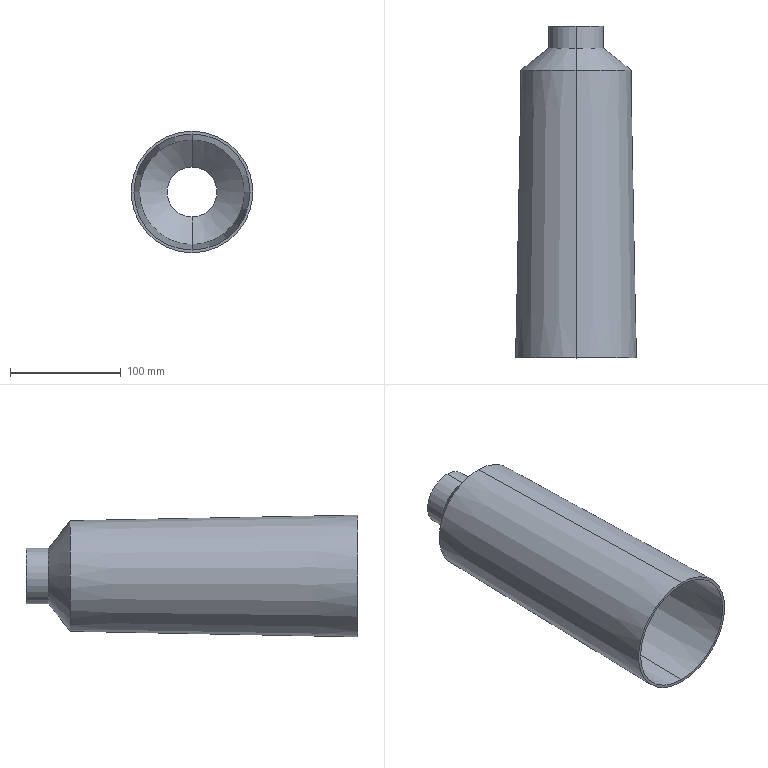Part | SolidWorks | features Revolution 1, Shell 1 | 1 solid | 14 faces | box 110 x 300 x 110 mm | volume 234806 mm3 | cone 8 | cylinder 4 | plane 2 | commonest cylinder face diameters 45 x2 50 x2
STEP:
#1=CARTESIAN_POINT('',(0.,258.78,47.523));
#2=VERTEX_POINT('',#1);
#3=CARTESIAN_POINT('',(0.,258.78,-47.523));
#4=VERTEX_POINT('',#3);
#5=CARTESIAN_POINT('',(0.,258.78,0.));
#6=DIRECTION('',(0.,-1.,0.));
#7=DIRECTION('',(0.,0.,-1.));
#8=AXIS2_PLACEMENT_3D('',#5,#6,#7);
#9=CIRCLE('',#8,47.523);
#10=EDGE_CURVE('',#2,#4,#9,.T.);
#11=ORIENTED_EDGE('',*,*,#10,.F.);
#12=CARTESIAN_POINT('',(0.,0.,52.5));
#13=VERTEX_POINT('',#12);
#14=CARTESIAN_POINT('',(0.,-0.04807,52.5));
#15=DIRECTION('',(0.,-0.9998,0.01923));
#16=VECTOR('',#15,1000.);
#17=LINE('',#14,#16);
#18=EDGE_CURVE('',#2,#13,#17,.T.);
#19=ORIENTED_EDGE('',*,*,#18,.T.);
#20=CARTESIAN_POINT('',(0.,0.,-52.5));
#21=VERTEX_POINT('',#20);
#22=CARTESIAN_POINT('',(0.,0.,0.));
#23=DIRECTION('',(0.,-1.,0.));
#24=DIRECTION('',(0.,0.,-1.));
#25=AXIS2_PLACEMENT_3D('',#22,#23,#24);
#26=CIRCLE('',#25,52.5);
#27=EDGE_CURVE('',#13,#21,#26,.T.);
#28=ORIENTED_EDGE('',*,*,#27,.T.);
#29=CARTESIAN_POINT('',(0.,-0.04807,-52.5));
#30=DIRECTION('',(0.,-0.9998,-0.01923));
#31=VECTOR('',#30,1000.);
#32=LINE('',#29,#31);
#33=EDGE_CURVE('',#4,#21,#32,.T.);
#34=ORIENTED_EDGE('',*,*,#33,.F.);
#35=EDGE_LOOP('',(#11,#19,#28,#34));
#36=FACE_OUTER_BOUND('',#35,.T.);
#37=CARTESIAN_POINT('',(0.,-0.04807,0.));
#38=DIRECTION('',(0.,-1.,0.));
#39=DIRECTION('',(0.,0.,-1.));
#40=AXIS2_PLACEMENT_3D('',#37,#38,#39);
#41=CONICAL_SURFACE('',#40,52.5,0.01923);
#42=ADVANCED_FACE('',(#36),#41,.F.);
#43=CARTESIAN_POINT('',(0.,278.798,22.5));
#44=VERTEX_POINT('',#43);
#45=CARTESIAN_POINT('',(0.,278.798,-22.5));
#46=VERTEX_POINT('',#45);
#47=CARTESIAN_POINT('',(0.,278.798,0.));
#48=DIRECTION('',(0.,-1.,0.));
#49=DIRECTION('',(0.,0.,-1.));
#50=AXIS2_PLACEMENT_3D('',#47,#48,#49);
#51=CIRCLE('',#50,22.5);
#52=EDGE_CURVE('',#44,#46,#51,.T.);
#53=ORIENTED_EDGE('',*,*,#52,.F.);
#54=CARTESIAN_POINT('',(0.,258.048,48.438));
#55=DIRECTION('',(0.,-0.6247,0.7809));
#56=VECTOR('',#55,1000.);
#57=LINE('',#54,#56);
#58=EDGE_CURVE('',#44,#2,#57,.T.);
#59=ORIENTED_EDGE('',*,*,#58,.T.);
#60=ORIENTED_EDGE('',*,*,#10,.T.);
#61=CARTESIAN_POINT('',(0.,258.048,-48.438));
#62=DIRECTION('',(0.,-0.6247,-0.7809));
#63=VECTOR('',#62,1000.);
#64=LINE('',#61,#63);
#65=EDGE_CURVE('',#46,#4,#64,.T.);
#66=ORIENTED_EDGE('',*,*,#65,.F.);
#67=EDGE_LOOP('',(#53,#59,#60,#66));
#68=FACE_OUTER_BOUND('',#67,.T.);
#69=CARTESIAN_POINT('',(0.,258.048,0.));
#70=DIRECTION('',(0.,-1.,0.));
#71=DIRECTION('',(0.,0.,-1.));
#72=AXIS2_PLACEMENT_3D('',#69,#70,#71);
#73=CONICAL_SURFACE('',#72,48.438,0.8961);
#74=ADVANCED_FACE('',(#68),#73,.F.);
#75=CARTESIAN_POINT('',(0.,300.,22.5));
#76=VERTEX_POINT('',#75);
#77=CARTESIAN_POINT('',(0.,300.,-22.5));
#78=VERTEX_POINT('',#77);
#79=CARTESIAN_POINT('',(0.,300.,0.));
#80=DIRECTION('',(0.,-1.,0.));
#81=DIRECTION('',(0.,0.,1.));
#82=AXIS2_PLACEMENT_3D('',#79,#80,#81);
#83=CIRCLE('',#82,22.5);
#84=EDGE_CURVE('',#76,#78,#83,.T.);
#85=ORIENTED_EDGE('',*,*,#84,.F.);
#86=CARTESIAN_POINT('',(0.,0.,22.5));
#87=DIRECTION('',(0.,-1.,0.));
#88=VECTOR('',#87,1000.);
#89=LINE('',#86,#88);
#90=EDGE_CURVE('',#76,#44,#89,.T.);
#91=ORIENTED_EDGE('',*,*,#90,.T.);
#92=ORIENTED_EDGE('',*,*,#52,.T.);
#93=CARTESIAN_POINT('',(0.,0.,-22.5));
#94=DIRECTION('',(0.,-1.,0.));
#95=VECTOR('',#94,1000.);
#96=LINE('',#93,#95);
#97=EDGE_CURVE('',#78,#46,#96,.T.);
#98=ORIENTED_EDGE('',*,*,#97,.F.);
#99=EDGE_LOOP('',(#85,#91,#92,#98));
#100=FACE_OUTER_BOUND('',#99,.T.);
#101=CARTESIAN_POINT('',(0.,0.,0.));
#102=DIRECTION('',(0.,-1.,0.));
#103=DIRECTION('',(0.,0.,-1.));
#104=AXIS2_PLACEMENT_3D('',#101,#102,#103);
#105=CYLINDRICAL_SURFACE('',#104,22.5);
#106=ADVANCED_FACE('',(#100),#105,.F.);
#107=CARTESIAN_POINT('',(0.,260.,-50.));
#108=VERTEX_POINT('',#107);
#109=CARTESIAN_POINT('',(0.,260.,50.));
#110=VERTEX_POINT('',#109);
#111=CARTESIAN_POINT('',(0.,260.,0.));
#112=DIRECTION('',(0.,-1.,0.));
#113=DIRECTION('',(0.,0.,-1.));
#114=AXIS2_PLACEMENT_3D('',#111,#112,#113);
#115=CIRCLE('',#114,50.);
#116=EDGE_CURVE('',#108,#110,#115,.T.);
#117=ORIENTED_EDGE('',*,*,#116,.T.);
#118=CARTESIAN_POINT('',(0.,0.,55.));
#119=VERTEX_POINT('',#118);
#120=CARTESIAN_POINT('',(0.,0.,55.));
#121=DIRECTION('',(0.,-0.9998,0.01923));
#122=VECTOR('',#121,1000.);
#123=LINE('',#120,#122);
#124=EDGE_CURVE('',#110,#119,#123,.T.);
#125=ORIENTED_EDGE('',*,*,#124,.T.);
#126=CARTESIAN_POINT('',(0.,0.,-55.));
#127=VERTEX_POINT('',#126);
#128=CARTESIAN_POINT('',(0.,0.,0.));
#129=DIRECTION('',(0.,-1.,0.));
#130=DIRECTION('',(0.,0.,-1.));
#131=AXIS2_PLACEMENT_3D('',#128,#129,#130);
#132=CIRCLE('',#131,55.);
#133=EDGE_CURVE('',#127,#119,#132,.T.);
#134=ORIENTED_EDGE('',*,*,#133,.F.);
#135=CARTESIAN_POINT('',(0.,0.,-55.));
#136=DIRECTION('',(0.,-0.9998,-0.01923));
#137=VECTOR('',#136,1000.);
#138=LINE('',#135,#137);
#139=EDGE_CURVE('',#108,#127,#138,.T.);
#140=ORIENTED_EDGE('',*,*,#139,.F.);
#141=EDGE_LOOP('',(#117,#125,#134,#140));
#142=FACE_OUTER_BOUND('',#141,.T.);
#143=CARTESIAN_POINT('',(0.,0.,0.));
#144=DIRECTION('',(0.,-1.,0.));
#145=DIRECTION('',(0.,0.,-1.));
#146=AXIS2_PLACEMENT_3D('',#143,#144,#145);
#147=CONICAL_SURFACE('',#146,55.,0.01923);
#148=ADVANCED_FACE('',(#142),#147,.T.);
#149=CARTESIAN_POINT('',(0.,280.,-25.));
#150=VERTEX_POINT('',#149);
#151=CARTESIAN_POINT('',(0.,280.,25.));
#152=VERTEX_POINT('',#151);
#153=CARTESIAN_POINT('',(0.,280.,0.));
#154=DIRECTION('',(0.,-1.,0.));
#155=DIRECTION('',(0.,0.,-1.));
#156=AXIS2_PLACEMENT_3D('',#153,#154,#155);
#157=CIRCLE('',#156,25.);
#158=EDGE_CURVE('',#150,#152,#157,.T.);
#159=ORIENTED_EDGE('',*,*,#158,.T.);
#160=CARTESIAN_POINT('',(0.,260.,50.));
#161=DIRECTION('',(0.,-0.6247,0.7809));
#162=VECTOR('',#161,1000.);
#163=LINE('',#160,#162);
#164=EDGE_CURVE('',#152,#110,#163,.T.);
#165=ORIENTED_EDGE('',*,*,#164,.T.);
#166=ORIENTED_EDGE('',*,*,#116,.F.);
#167=CARTESIAN_POINT('',(0.,260.,-50.));
#168=DIRECTION('',(0.,-0.6247,-0.7809));
#169=VECTOR('',#168,1000.);
#170=LINE('',#167,#169);
#171=EDGE_CURVE('',#150,#108,#170,.T.);
#172=ORIENTED_EDGE('',*,*,#171,.F.);
#173=EDGE_LOOP('',(#159,#165,#166,#172));
#174=FACE_OUTER_BOUND('',#173,.T.);
#175=CARTESIAN_POINT('',(0.,260.,0.));
#176=DIRECTION('',(0.,-1.,0.));
#177=DIRECTION('',(0.,0.,-1.));
#178=AXIS2_PLACEMENT_3D('',#175,#176,#177);
#179=CONICAL_SURFACE('',#178,50.,0.8961);
#180=ADVANCED_FACE('',(#174),#179,.T.);
#181=CARTESIAN_POINT('',(0.,300.,-25.));
#182=VERTEX_POINT('',#181);
#183=CARTESIAN_POINT('',(0.,300.,25.));
#184=VERTEX_POINT('',#183);
#185=CARTESIAN_POINT('',(0.,300.,0.));
#186=DIRECTION('',(0.,-1.,0.));
#187=DIRECTION('',(0.,0.,-1.));
#188=AXIS2_PLACEMENT_3D('',#185,#186,#187);
#189=CIRCLE('',#188,25.);
#190=EDGE_CURVE('',#182,#184,#189,.T.);
#191=ORIENTED_EDGE('',*,*,#190,.T.);
#192=CARTESIAN_POINT('',(0.,0.,25.));
#193=DIRECTION('',(0.,-1.,0.));
#194=VECTOR('',#193,1000.);
#195=LINE('',#192,#194);
#196=EDGE_CURVE('',#184,#152,#195,.T.);
#197=ORIENTED_EDGE('',*,*,#196,.T.);
#198=ORIENTED_EDGE('',*,*,#158,.F.);
#199=CARTESIAN_POINT('',(0.,0.,-25.));
#200=DIRECTION('',(0.,-1.,0.));
#201=VECTOR('',#200,1000.);
#202=LINE('',#199,#201);
#203=EDGE_CURVE('',#182,#150,#202,.T.);
#204=ORIENTED_EDGE('',*,*,#203,.F.);
#205=EDGE_LOOP('',(#191,#197,#198,#204));
#206=FACE_OUTER_BOUND('',#205,.T.);
#207=CARTESIAN_POINT('',(0.,0.,0.));
#208=DIRECTION('',(0.,-1.,0.));
#209=DIRECTION('',(0.,0.,-1.));
#210=AXIS2_PLACEMENT_3D('',#207,#208,#209);
#211=CYLINDRICAL_SURFACE('',#210,25.);
#212=ADVANCED_FACE('',(#206),#211,.T.);
#213=CARTESIAN_POINT('',(0.,0.,0.));
#214=DIRECTION('',(0.,-1.,0.));
#215=DIRECTION('',(0.,0.,-1.));
#216=AXIS2_PLACEMENT_3D('',#213,#214,#215);
#217=CIRCLE('',#216,52.5);
#218=EDGE_CURVE('',#21,#13,#217,.T.);
#219=ORIENTED_EDGE('',*,*,#218,.F.);
#220=ORIENTED_EDGE('',*,*,#27,.F.);
#221=EDGE_LOOP('',(#219,#220));
#222=FACE_BOUND('',#221,.T.);
#223=ORIENTED_EDGE('',*,*,#133,.T.);
#224=CARTESIAN_POINT('',(0.,0.,0.));
#225=DIRECTION('',(0.,-1.,0.));
#226=DIRECTION('',(0.,0.,-1.));
#227=AXIS2_PLACEMENT_3D('',#224,#225,#226);
#228=CIRCLE('',#227,55.);
#229=EDGE_CURVE('',#119,#127,#228,.T.);
#230=ORIENTED_EDGE('',*,*,#229,.T.);
#231=EDGE_LOOP('',(#223,#230));
#232=FACE_OUTER_BOUND('',#231,.T.);
#233=CARTESIAN_POINT('',(55.,0.,0.));
#234=DIRECTION('',(0.,-1.,0.));
#235=DIRECTION('',(0.,0.,-1.));
#236=AXIS2_PLACEMENT_3D('',#233,#234,#235);
#237=PLANE('',#236);
#238=ADVANCED_FACE('',(#222,#232),#237,.T.);
#239=CARTESIAN_POINT('',(0.,300.,0.));
#240=DIRECTION('',(0.,-1.,0.));
#241=DIRECTION('',(0.,0.,1.));
#242=AXIS2_PLACEMENT_3D('',#239,#240,#241);
#243=CIRCLE('',#242,22.5);
#244=EDGE_CURVE('',#78,#76,#243,.T.);
#245=ORIENTED_EDGE('',*,*,#244,.T.);
#246=ORIENTED_EDGE('',*,*,#84,.T.);
#247=EDGE_LOOP('',(#245,#246));
#248=FACE_BOUND('',#247,.T.);
#249=ORIENTED_EDGE('',*,*,#190,.F.);
#250=CARTESIAN_POINT('',(0.,300.,0.));
#251=DIRECTION('',(0.,-1.,0.));
#252=DIRECTION('',(0.,0.,-1.));
#253=AXIS2_PLACEMENT_3D('',#250,#251,#252);
#254=CIRCLE('',#253,25.);
#255=EDGE_CURVE('',#184,#182,#254,.T.);
#256=ORIENTED_EDGE('',*,*,#255,.F.);
#257=EDGE_LOOP('',(#249,#256));
#258=FACE_OUTER_BOUND('',#257,.T.);
#259=CARTESIAN_POINT('',(0.,300.,0.));
#260=DIRECTION('',(0.,1.,0.));
#261=DIRECTION('',(0.,0.,1.));
#262=AXIS2_PLACEMENT_3D('',#259,#260,#261);
#263=PLANE('',#262);
#264=ADVANCED_FACE('',(#248,#258),#263,.T.);
#265=ORIENTED_EDGE('',*,*,#196,.F.);
#266=ORIENTED_EDGE('',*,*,#255,.T.);
#267=ORIENTED_EDGE('',*,*,#203,.T.);
#268=CARTESIAN_POINT('',(0.,280.,0.));
#269=DIRECTION('',(0.,-1.,0.));
#270=DIRECTION('',(0.,0.,-1.));
#271=AXIS2_PLACEMENT_3D('',#268,#269,#270);
#272=CIRCLE('',#271,25.);
#273=EDGE_CURVE('',#152,#150,#272,.T.);
#274=ORIENTED_EDGE('',*,*,#273,.F.);
#275=EDGE_LOOP('',(#265,#266,#267,#274));
#276=FACE_OUTER_BOUND('',#275,.T.);
#277=CARTESIAN_POINT('',(0.,0.,0.));
#278=DIRECTION('',(0.,-1.,0.));
#279=DIRECTION('',(0.,0.,-1.));
#280=AXIS2_PLACEMENT_3D('',#277,#278,#279);
#281=CYLINDRICAL_SURFACE('',#280,25.);
#282=ADVANCED_FACE('',(#276),#281,.T.);
#283=ORIENTED_EDGE('',*,*,#164,.F.);
#284=ORIENTED_EDGE('',*,*,#273,.T.);
#285=ORIENTED_EDGE('',*,*,#171,.T.);
#286=CARTESIAN_POINT('',(0.,260.,0.));
#287=DIRECTION('',(0.,-1.,0.));
#288=DIRECTION('',(0.,0.,-1.));
#289=AXIS2_PLACEMENT_3D('',#286,#287,#288);
#290=CIRCLE('',#289,50.);
#291=EDGE_CURVE('',#110,#108,#290,.T.);
#292=ORIENTED_EDGE('',*,*,#291,.F.);
#293=EDGE_LOOP('',(#283,#284,#285,#292));
#294=FACE_OUTER_BOUND('',#293,.T.);
#295=CARTESIAN_POINT('',(0.,260.,0.));
#296=DIRECTION('',(0.,-1.,0.));
#297=DIRECTION('',(0.,0.,-1.));
#298=AXIS2_PLACEMENT_3D('',#295,#296,#297);
#299=CONICAL_SURFACE('',#298,50.,0.8961);
#300=ADVANCED_FACE('',(#294),#299,.T.);
#301=ORIENTED_EDGE('',*,*,#124,.F.);
#302=ORIENTED_EDGE('',*,*,#291,.T.);
#303=ORIENTED_EDGE('',*,*,#139,.T.);
#304=ORIENTED_EDGE('',*,*,#229,.F.);
#305=EDGE_LOOP('',(#301,#302,#303,#304));
#306=FACE_OUTER_BOUND('',#305,.T.);
#307=CARTESIAN_POINT('',(0.,0.,0.));
#308=DIRECTION('',(0.,-1.,0.));
#309=DIRECTION('',(0.,0.,-1.));
#310=AXIS2_PLACEMENT_3D('',#307,#308,#309);
#311=CONICAL_SURFACE('',#310,55.,0.01923);
#312=ADVANCED_FACE('',(#306),#311,.T.);
#313=ORIENTED_EDGE('',*,*,#90,.F.);
#314=ORIENTED_EDGE('',*,*,#244,.F.);
#315=ORIENTED_EDGE('',*,*,#97,.T.);
#316=CARTESIAN_POINT('',(0.,278.798,0.));
#317=DIRECTION('',(0.,-1.,0.));
#318=DIRECTION('',(0.,0.,-1.));
#319=AXIS2_PLACEMENT_3D('',#316,#317,#318);
#320=CIRCLE('',#319,22.5);
#321=EDGE_CURVE('',#46,#44,#320,.T.);
#322=ORIENTED_EDGE('',*,*,#321,.T.);
#323=EDGE_LOOP('',(#313,#314,#315,#322));
#324=FACE_OUTER_BOUND('',#323,.T.);
#325=CARTESIAN_POINT('',(0.,0.,0.));
#326=DIRECTION('',(0.,-1.,0.));
#327=DIRECTION('',(0.,0.,-1.));
#328=AXIS2_PLACEMENT_3D('',#325,#326,#327);
#329=CYLINDRICAL_SURFACE('',#328,22.5);
#330=ADVANCED_FACE('',(#324),#329,.F.);
#331=ORIENTED_EDGE('',*,*,#58,.F.);
#332=ORIENTED_EDGE('',*,*,#321,.F.);
#333=ORIENTED_EDGE('',*,*,#65,.T.);
#334=CARTESIAN_POINT('',(0.,258.78,0.));
#335=DIRECTION('',(0.,-1.,0.));
#336=DIRECTION('',(0.,0.,-1.));
#337=AXIS2_PLACEMENT_3D('',#334,#335,#336);
#338=CIRCLE('',#337,47.523);
#339=EDGE_CURVE('',#4,#2,#338,.T.);
#340=ORIENTED_EDGE('',*,*,#339,.T.);
#341=EDGE_LOOP('',(#331,#332,#333,#340));
#342=FACE_OUTER_BOUND('',#341,.T.);
#343=CARTESIAN_POINT('',(0.,258.048,0.));
#344=DIRECTION('',(0.,-1.,0.));
#345=DIRECTION('',(0.,0.,-1.));
#346=AXIS2_PLACEMENT_3D('',#343,#344,#345);
#347=CONICAL_SURFACE('',#346,48.438,0.8961);
#348=ADVANCED_FACE('',(#342),#347,.F.);
#349=ORIENTED_EDGE('',*,*,#18,.F.);
#350=ORIENTED_EDGE('',*,*,#339,.F.);
#351=ORIENTED_EDGE('',*,*,#33,.T.);
#352=ORIENTED_EDGE('',*,*,#218,.T.);
#353=EDGE_LOOP('',(#349,#350,#351,#352));
#354=FACE_OUTER_BOUND('',#353,.T.);
#355=CARTESIAN_POINT('',(0.,-0.04807,0.));
#356=DIRECTION('',(0.,-1.,0.));
#357=DIRECTION('',(0.,0.,-1.));
#358=AXIS2_PLACEMENT_3D('',#355,#356,#357);
#359=CONICAL_SURFACE('',#358,52.5,0.01923);
#360=ADVANCED_FACE('',(#354),#359,.F.);
#361=CLOSED_SHELL('',(#42,#74,#106,#148,#180,#212,#238,#264,#282,#300,#312,#330,#348,#360));
#362=MANIFOLD_SOLID_BREP('',#361);
#363=CARTESIAN_POINT('',(0.,0.,0.));
#364=DIRECTION('',(0.,0.,1.));
#365=DIRECTION('',(1.,0.,0.));
#366=AXIS2_PLACEMENT_3D('',#363,#364,#365);
#367=(LENGTH_UNIT()NAMED_UNIT(*)SI_UNIT(.MILLI.,.METRE.));
#368=UNCERTAINTY_MEASURE_WITH_UNIT(LENGTH_MEASURE(0.00001),#367,'','');
#369=(NAMED_UNIT(*)PLANE_ANGLE_UNIT()SI_UNIT($,.RADIAN.));
#370=(NAMED_UNIT(*)SI_UNIT($,.STERADIAN.)SOLID_ANGLE_UNIT());
#371=(GEOMETRIC_REPRESENTATION_CONTEXT(3)GLOBAL_UNCERTAINTY_ASSIGNED_CONTEXT((#368))GLOBAL_UNIT_ASSIGNED_CONTEXT((#367,#369,#370))REPRESENTATION_CONTEXT('',''));
#372=ADVANCED_BREP_SHAPE_REPRESENTATION('',(#362,#366),#371);